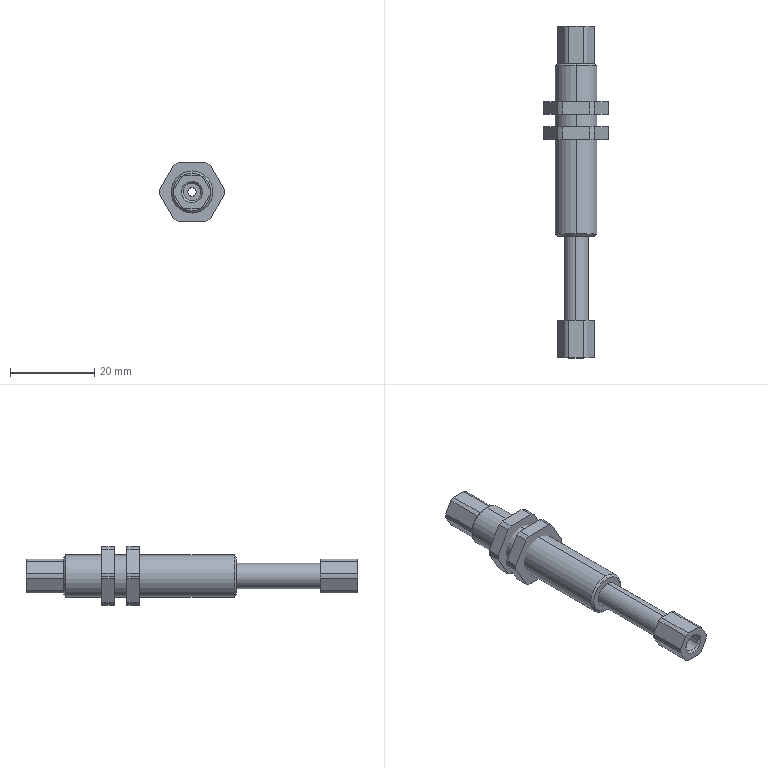Part | SolidWorks | features BaseBody 6 | 6 solids | 104 faces | box 15.5 x 79 x 14 mm | volume 4777 mm3 | cylinder 52 | plane 40 | cone 12 | commonest cylinder face diameters 15.5 x16 8.7 x12 4.13 x6 9 x4 2 x2 4.132 x2